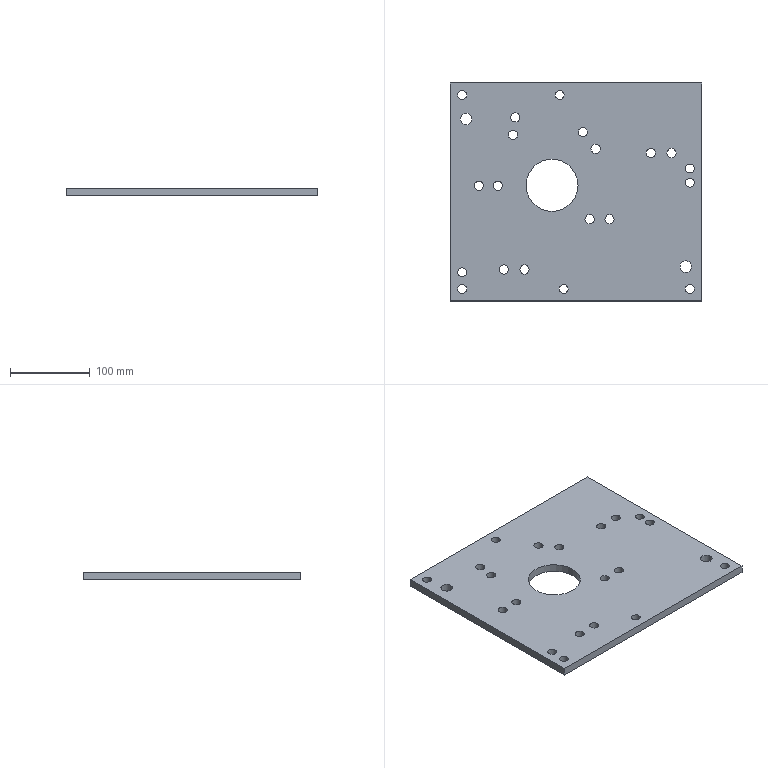Part | STEP file | lll_id3006_x_t | 1 solid | 29 faces | box 315 x 273 x 10 mm | volume 803171 mm3 | cylinder 23 | plane 6 | commonest cylinder face diameters 11.509 x12 11 x8 14.505 x2 65.2 x1
STEP:
#1=CARTESIAN_POINT('',(3327.121,-63.788,92.5));
#2=VERTEX_POINT('',#1);
#3=CARTESIAN_POINT('',(3321.367,-63.788,92.5));
#4=DIRECTION('',(0.,0.,1.));
#5=DIRECTION('',(1.,0.,0.));
#6=AXIS2_PLACEMENT_3D('',#3,#4,#5);
#7=CIRCLE('',#6,5.755);
#8=EDGE_CURVE('',#2,#2,#7,.T.);
#9=ORIENTED_EDGE('',*,*,#8,.F.);
#10=EDGE_LOOP('',(#9));
#11=FACE_BOUND('',#10,.T.);
#12=CARTESIAN_POINT('',(3315.612,-63.788,102.5));
#13=VERTEX_POINT('',#12);
#14=CARTESIAN_POINT('',(3321.367,-63.788,102.5));
#15=DIRECTION('',(0.,0.,-1.));
#16=DIRECTION('',(-1.,0.,0.));
#17=AXIS2_PLACEMENT_3D('',#14,#15,#16);
#18=CIRCLE('',#17,5.755);
#19=EDGE_CURVE('',#13,#13,#18,.T.);
#20=ORIENTED_EDGE('',*,*,#19,.F.);
#21=EDGE_LOOP('',(#20));
#22=FACE_BOUND('',#21,.T.);
#23=CARTESIAN_POINT('',(3321.367,-63.788,79.5));
#24=DIRECTION('',(0.,0.,1.));
#25=DIRECTION('',(1.,0.,0.));
#26=AXIS2_PLACEMENT_3D('',#23,#24,#25);
#27=CYLINDRICAL_SURFACE('',#26,5.755);
#28=ADVANCED_FACE('',(#11,#22),#27,.F.);
#29=CARTESIAN_POINT('',(3343.121,-84.788,92.5));
#30=VERTEX_POINT('',#29);
#31=CARTESIAN_POINT('',(3337.367,-84.788,92.5));
#32=DIRECTION('',(0.,0.,-1.));
#33=DIRECTION('',(1.,0.,0.));
#34=AXIS2_PLACEMENT_3D('',#31,#32,#33);
#35=CIRCLE('',#34,5.755);
#36=EDGE_CURVE('',#30,#30,#35,.T.);
#37=ORIENTED_EDGE('',*,*,#36,.T.);
#38=EDGE_LOOP('',(#37));
#39=FACE_BOUND('',#38,.T.);
#40=CARTESIAN_POINT('',(3331.612,-84.788,102.5));
#41=VERTEX_POINT('',#40);
#42=CARTESIAN_POINT('',(3337.367,-84.788,102.5));
#43=DIRECTION('',(0.,0.,-1.));
#44=DIRECTION('',(-1.,0.,0.));
#45=AXIS2_PLACEMENT_3D('',#42,#43,#44);
#46=CIRCLE('',#45,5.755);
#47=EDGE_CURVE('',#41,#41,#46,.T.);
#48=ORIENTED_EDGE('',*,*,#47,.F.);
#49=EDGE_LOOP('',(#48));
#50=FACE_BOUND('',#49,.T.);
#51=CARTESIAN_POINT('',(3337.367,-84.788,79.5));
#52=DIRECTION('',(0.,0.,1.));
#53=DIRECTION('',(1.,0.,0.));
#54=AXIS2_PLACEMENT_3D('',#51,#52,#53);
#55=CYLINDRICAL_SURFACE('',#54,5.755);
#56=ADVANCED_FACE('',(#39,#50),#55,.F.);
#57=CARTESIAN_POINT('',(3168.115,-47.288,102.5));
#58=VERTEX_POINT('',#57);
#59=CARTESIAN_POINT('',(3175.367,-47.288,102.5));
#60=DIRECTION('',(0.,0.,-1.));
#61=DIRECTION('',(-1.,0.,0.));
#62=AXIS2_PLACEMENT_3D('',#59,#60,#61);
#63=CIRCLE('',#62,7.253);
#64=EDGE_CURVE('',#58,#58,#63,.T.);
#65=ORIENTED_EDGE('',*,*,#64,.F.);
#66=EDGE_LOOP('',(#65));
#67=FACE_BOUND('',#66,.T.);
#68=CARTESIAN_POINT('',(3182.62,-47.288,92.5));
#69=VERTEX_POINT('',#68);
#70=CARTESIAN_POINT('',(3175.367,-47.288,92.5));
#71=DIRECTION('',(0.,0.,1.));
#72=DIRECTION('',(1.,0.,0.));
#73=AXIS2_PLACEMENT_3D('',#70,#71,#72);
#74=CIRCLE('',#73,7.253);
#75=EDGE_CURVE('',#69,#69,#74,.T.);
#76=ORIENTED_EDGE('',*,*,#75,.F.);
#77=EDGE_LOOP('',(#76));
#78=FACE_BOUND('',#77,.T.);
#79=CARTESIAN_POINT('',(3175.367,-47.288,92.5));
#80=DIRECTION('',(0.,0.,1.));
#81=DIRECTION('',(1.,0.,0.));
#82=AXIS2_PLACEMENT_3D('',#79,#80,#81);
#83=CYLINDRICAL_SURFACE('',#82,7.253);
#84=ADVANCED_FACE('',(#67,#78),#83,.F.);
#85=CARTESIAN_POINT('',(3324.113,-172.788,102.5));
#86=VERTEX_POINT('',#85);
#87=CARTESIAN_POINT('',(3329.867,-172.788,102.5));
#88=DIRECTION('',(0.,0.,1.));
#89=DIRECTION('',(-1.,0.,0.));
#90=AXIS2_PLACEMENT_3D('',#87,#88,#89);
#91=CIRCLE('',#90,5.755);
#92=EDGE_CURVE('',#86,#86,#91,.T.);
#93=ORIENTED_EDGE('',*,*,#92,.T.);
#94=EDGE_LOOP('',(#93));
#95=FACE_BOUND('',#94,.T.);
#96=CARTESIAN_POINT('',(3335.622,-172.788,92.5));
#97=VERTEX_POINT('',#96);
#98=CARTESIAN_POINT('',(3329.867,-172.788,92.5));
#99=DIRECTION('',(0.,0.,1.));
#100=DIRECTION('',(1.,0.,0.));
#101=AXIS2_PLACEMENT_3D('',#98,#99,#100);
#102=CIRCLE('',#101,5.755);
#103=EDGE_CURVE('',#97,#97,#102,.T.);
#104=ORIENTED_EDGE('',*,*,#103,.F.);
#105=EDGE_LOOP('',(#104));
#106=FACE_BOUND('',#105,.T.);
#107=CARTESIAN_POINT('',(3329.867,-172.788,92.5));
#108=DIRECTION('',(0.,0.,1.));
#109=DIRECTION('',(1.,0.,0.));
#110=AXIS2_PLACEMENT_3D('',#107,#108,#109);
#111=CYLINDRICAL_SURFACE('',#110,5.755);
#112=ADVANCED_FACE('',(#95,#106),#111,.F.);
#113=CARTESIAN_POINT('',(3216.612,-235.788,102.5));
#114=VERTEX_POINT('',#113);
#115=CARTESIAN_POINT('',(3222.367,-235.788,102.5));
#116=DIRECTION('',(0.,0.,-1.));
#117=DIRECTION('',(-1.,0.,0.));
#118=AXIS2_PLACEMENT_3D('',#115,#116,#117);
#119=CIRCLE('',#118,5.755);
#120=EDGE_CURVE('',#114,#114,#119,.T.);
#121=ORIENTED_EDGE('',*,*,#120,.F.);
#122=EDGE_LOOP('',(#121));
#123=FACE_BOUND('',#122,.T.);
#124=CARTESIAN_POINT('',(3228.121,-235.788,92.5));
#125=VERTEX_POINT('',#124);
#126=CARTESIAN_POINT('',(3222.367,-235.788,92.5));
#127=DIRECTION('',(0.,0.,1.));
#128=DIRECTION('',(1.,0.,0.));
#129=AXIS2_PLACEMENT_3D('',#126,#127,#128);
#130=CIRCLE('',#129,5.755);
#131=EDGE_CURVE('',#125,#125,#130,.T.);
#132=ORIENTED_EDGE('',*,*,#131,.F.);
#133=EDGE_LOOP('',(#132));
#134=FACE_BOUND('',#133,.T.);
#135=CARTESIAN_POINT('',(3222.367,-235.788,92.5));
#136=DIRECTION('',(0.,0.,1.));
#137=DIRECTION('',(1.,0.,0.));
#138=AXIS2_PLACEMENT_3D('',#135,#136,#137);
#139=CYLINDRICAL_SURFACE('',#138,5.755);
#140=ADVANCED_FACE('',(#123,#134),#139,.F.);
#141=CARTESIAN_POINT('',(3209.245,-131.,102.5));
#142=VERTEX_POINT('',#141);
#143=CARTESIAN_POINT('',(3215.,-131.,102.5));
#144=DIRECTION('',(0.,0.,1.));
#145=DIRECTION('',(-1.,0.,0.));
#146=AXIS2_PLACEMENT_3D('',#143,#144,#145);
#147=CIRCLE('',#146,5.755);
#148=EDGE_CURVE('',#142,#142,#147,.T.);
#149=ORIENTED_EDGE('',*,*,#148,.T.);
#150=EDGE_LOOP('',(#149));
#151=FACE_BOUND('',#150,.T.);
#152=CARTESIAN_POINT('',(3220.755,-131.,92.5));
#153=VERTEX_POINT('',#152);
#154=CARTESIAN_POINT('',(3215.,-131.,92.5));
#155=DIRECTION('',(0.,0.,1.));
#156=DIRECTION('',(1.,0.,0.));
#157=AXIS2_PLACEMENT_3D('',#154,#155,#156);
#158=CIRCLE('',#157,5.755);
#159=EDGE_CURVE('',#153,#153,#158,.T.);
#160=ORIENTED_EDGE('',*,*,#159,.F.);
#161=EDGE_LOOP('',(#160));
#162=FACE_BOUND('',#161,.T.);
#163=CARTESIAN_POINT('',(3215.,-131.,92.5));
#164=DIRECTION('',(0.,0.,1.));
#165=DIRECTION('',(1.,0.,0.));
#166=AXIS2_PLACEMENT_3D('',#163,#164,#165);
#167=CYLINDRICAL_SURFACE('',#166,5.755);
#168=ADVANCED_FACE('',(#151,#162),#167,.F.);
#169=CARTESIAN_POINT('',(3400.746,-90.,102.5));
#170=VERTEX_POINT('',#169);
#171=CARTESIAN_POINT('',(3406.5,-90.,102.5));
#172=DIRECTION('',(0.,0.,1.));
#173=DIRECTION('',(-1.,0.,0.));
#174=AXIS2_PLACEMENT_3D('',#171,#172,#173);
#175=CIRCLE('',#174,5.755);
#176=EDGE_CURVE('',#170,#170,#175,.T.);
#177=ORIENTED_EDGE('',*,*,#176,.T.);
#178=EDGE_LOOP('',(#177));
#179=FACE_BOUND('',#178,.T.);
#180=CARTESIAN_POINT('',(3412.255,-90.,92.5));
#181=VERTEX_POINT('',#180);
#182=CARTESIAN_POINT('',(3406.5,-90.,92.5));
#183=DIRECTION('',(0.,0.,1.));
#184=DIRECTION('',(1.,0.,0.));
#185=AXIS2_PLACEMENT_3D('',#182,#183,#184);
#186=CIRCLE('',#185,5.755);
#187=EDGE_CURVE('',#181,#181,#186,.T.);
#188=ORIENTED_EDGE('',*,*,#187,.F.);
#189=EDGE_LOOP('',(#188));
#190=FACE_BOUND('',#189,.T.);
#191=CARTESIAN_POINT('',(3406.5,-90.,92.5));
#192=DIRECTION('',(0.,0.,1.));
#193=DIRECTION('',(1.,0.,0.));
#194=AXIS2_PLACEMENT_3D('',#191,#192,#193);
#195=CYLINDRICAL_SURFACE('',#194,5.755);
#196=ADVANCED_FACE('',(#179,#190),#195,.F.);
#197=CARTESIAN_POINT('',(3228.222,-67.288,102.5));
#198=VERTEX_POINT('',#197);
#199=CARTESIAN_POINT('',(3233.977,-67.288,102.5));
#200=DIRECTION('',(0.,0.,1.));
#201=DIRECTION('',(-1.,0.,0.));
#202=AXIS2_PLACEMENT_3D('',#199,#200,#201);
#203=CIRCLE('',#202,5.755);
#204=EDGE_CURVE('',#198,#198,#203,.T.);
#205=ORIENTED_EDGE('',*,*,#204,.T.);
#206=EDGE_LOOP('',(#205));
#207=FACE_BOUND('',#206,.T.);
#208=CARTESIAN_POINT('',(3239.731,-67.288,92.5));
#209=VERTEX_POINT('',#208);
#210=CARTESIAN_POINT('',(3233.977,-67.288,92.5));
#211=DIRECTION('',(0.,0.,1.));
#212=DIRECTION('',(1.,0.,0.));
#213=AXIS2_PLACEMENT_3D('',#210,#211,#212);
#214=CIRCLE('',#213,5.755);
#215=EDGE_CURVE('',#209,#209,#214,.T.);
#216=ORIENTED_EDGE('',*,*,#215,.F.);
#217=EDGE_LOOP('',(#216));
#218=FACE_BOUND('',#217,.T.);
#219=CARTESIAN_POINT('',(3233.977,-67.288,92.5));
#220=DIRECTION('',(0.,0.,1.));
#221=DIRECTION('',(1.,0.,0.));
#222=AXIS2_PLACEMENT_3D('',#219,#220,#221);
#223=CYLINDRICAL_SURFACE('',#222,5.755);
#224=ADVANCED_FACE('',(#207,#218),#223,.F.);
#225=CARTESIAN_POINT('',(3449.867,-127.288,102.5));
#226=VERTEX_POINT('',#225);
#227=CARTESIAN_POINT('',(3455.367,-127.288,102.5));
#228=DIRECTION('',(0.,0.,-1.));
#229=DIRECTION('',(-1.,0.,0.));
#230=AXIS2_PLACEMENT_3D('',#227,#228,#229);
#231=CIRCLE('',#230,5.5);
#232=EDGE_CURVE('',#226,#226,#231,.T.);
#233=ORIENTED_EDGE('',*,*,#232,.F.);
#234=EDGE_LOOP('',(#233));
#235=FACE_BOUND('',#234,.T.);
#236=CARTESIAN_POINT('',(3460.867,-127.288,92.5));
#237=VERTEX_POINT('',#236);
#238=CARTESIAN_POINT('',(3455.367,-127.288,92.5));
#239=DIRECTION('',(0.,0.,1.));
#240=DIRECTION('',(1.,0.,0.));
#241=AXIS2_PLACEMENT_3D('',#238,#239,#240);
#242=CIRCLE('',#241,5.5);
#243=EDGE_CURVE('',#237,#237,#242,.T.);
#244=ORIENTED_EDGE('',*,*,#243,.F.);
#245=EDGE_LOOP('',(#244));
#246=FACE_BOUND('',#245,.T.);
#247=CARTESIAN_POINT('',(3455.367,-127.288,92.5));
#248=DIRECTION('',(0.,0.,-1.));
#249=DIRECTION('',(1.,0.,0.));
#250=AXIS2_PLACEMENT_3D('',#247,#248,#249);
#251=CYLINDRICAL_SURFACE('',#250,5.5);
#252=ADVANCED_FACE('',(#235,#246),#251,.F.);
#253=CARTESIAN_POINT('',(3164.867,-239.288,102.5));
#254=VERTEX_POINT('',#253);
#255=CARTESIAN_POINT('',(3170.367,-239.288,102.5));
#256=DIRECTION('',(0.,0.,-1.));
#257=DIRECTION('',(-1.,0.,0.));
#258=AXIS2_PLACEMENT_3D('',#255,#256,#257);
#259=CIRCLE('',#258,5.5);
#260=EDGE_CURVE('',#254,#254,#259,.T.);
#261=ORIENTED_EDGE('',*,*,#260,.F.);
#262=EDGE_LOOP('',(#261));
#263=FACE_BOUND('',#262,.T.);
#264=CARTESIAN_POINT('',(3175.867,-239.288,92.5));
#265=VERTEX_POINT('',#264);
#266=CARTESIAN_POINT('',(3170.367,-239.288,92.5));
#267=DIRECTION('',(0.,0.,1.));
#268=DIRECTION('',(1.,0.,0.));
#269=AXIS2_PLACEMENT_3D('',#266,#267,#268);
#270=CIRCLE('',#269,5.5);
#271=EDGE_CURVE('',#265,#265,#270,.T.);
#272=ORIENTED_EDGE('',*,*,#271,.F.);
#273=EDGE_LOOP('',(#272));
#274=FACE_BOUND('',#273,.T.);
#275=CARTESIAN_POINT('',(3170.367,-239.288,92.5));
#276=DIRECTION('',(0.,0.,-1.));
#277=DIRECTION('',(1.,0.,0.));
#278=AXIS2_PLACEMENT_3D('',#275,#276,#277);
#279=CYLINDRICAL_SURFACE('',#278,5.5);
#280=ADVANCED_FACE('',(#263,#274),#279,.F.);
#281=CARTESIAN_POINT('',(3449.867,-109.288,102.5));
#282=VERTEX_POINT('',#281);
#283=CARTESIAN_POINT('',(3455.367,-109.288,102.5));
#284=DIRECTION('',(0.,0.,1.));
#285=DIRECTION('',(-1.,0.,0.));
#286=AXIS2_PLACEMENT_3D('',#283,#284,#285);
#287=CIRCLE('',#286,5.5);
#288=EDGE_CURVE('',#282,#282,#287,.T.);
#289=ORIENTED_EDGE('',*,*,#288,.T.);
#290=EDGE_LOOP('',(#289));
#291=FACE_BOUND('',#290,.T.);
#292=CARTESIAN_POINT('',(3449.867,-109.288,92.5));
#293=VERTEX_POINT('',#292);
#294=CARTESIAN_POINT('',(3455.367,-109.288,92.5));
#295=DIRECTION('',(0.,0.,1.));
#296=DIRECTION('',(-1.,0.,0.));
#297=AXIS2_PLACEMENT_3D('',#294,#295,#296);
#298=CIRCLE('',#297,5.5);
#299=EDGE_CURVE('',#293,#293,#298,.T.);
#300=ORIENTED_EDGE('',*,*,#299,.F.);
#301=EDGE_LOOP('',(#300));
#302=FACE_BOUND('',#301,.T.);
#303=CARTESIAN_POINT('',(3455.367,-109.288,92.5));
#304=DIRECTION('',(0.,0.,-1.));
#305=DIRECTION('',(1.,0.,0.));
#306=AXIS2_PLACEMENT_3D('',#303,#304,#305);
#307=CYLINDRICAL_SURFACE('',#306,5.5);
#308=ADVANCED_FACE('',(#291,#302),#307,.F.);
#309=CARTESIAN_POINT('',(3164.867,-17.288,102.5));
#310=VERTEX_POINT('',#309);
#311=CARTESIAN_POINT('',(3170.367,-17.288,102.5));
#312=DIRECTION('',(0.,0.,1.));
#313=DIRECTION('',(-1.,0.,0.));
#314=AXIS2_PLACEMENT_3D('',#311,#312,#313);
#315=CIRCLE('',#314,5.5);
#316=EDGE_CURVE('',#310,#310,#315,.T.);
#317=ORIENTED_EDGE('',*,*,#316,.T.);
#318=EDGE_LOOP('',(#317));
#319=FACE_BOUND('',#318,.T.);
#320=CARTESIAN_POINT('',(3164.867,-17.288,92.5));
#321=VERTEX_POINT('',#320);
#322=CARTESIAN_POINT('',(3170.367,-17.288,92.5));
#323=DIRECTION('',(0.,0.,1.));
#324=DIRECTION('',(-1.,0.,0.));
#325=AXIS2_PLACEMENT_3D('',#322,#323,#324);
#326=CIRCLE('',#325,5.5);
#327=EDGE_CURVE('',#321,#321,#326,.T.);
#328=ORIENTED_EDGE('',*,*,#327,.F.);
#329=EDGE_LOOP('',(#328));
#330=FACE_BOUND('',#329,.T.);
#331=CARTESIAN_POINT('',(3170.367,-17.288,92.5));
#332=DIRECTION('',(0.,0.,-1.));
#333=DIRECTION('',(1.,0.,0.));
#334=AXIS2_PLACEMENT_3D('',#331,#332,#333);
#335=CYLINDRICAL_SURFACE('',#334,5.5);
#336=ADVANCED_FACE('',(#319,#330),#335,.F.);
#337=CARTESIAN_POINT('',(3155.367,-275.288,102.5));
#338=VERTEX_POINT('',#337);
#339=CARTESIAN_POINT('',(3155.367,-275.288,92.5));
#340=VERTEX_POINT('',#339);
#341=CARTESIAN_POINT('',(3155.367,-275.288,92.5));
#342=DIRECTION('',(0.,0.,-1.));
#343=VECTOR('',#342,1.);
#344=LINE('',#341,#343);
#345=EDGE_CURVE('',#338,#340,#344,.T.);
#346=ORIENTED_EDGE('',*,*,#345,.F.);
#347=CARTESIAN_POINT('',(3155.367,-2.288,102.5));
#348=VERTEX_POINT('',#347);
#349=CARTESIAN_POINT('',(3155.367,-166.13,102.5));
#350=DIRECTION('',(0.,-1.,0.));
#351=VECTOR('',#350,1.);
#352=LINE('',#349,#351);
#353=EDGE_CURVE('',#348,#338,#352,.T.);
#354=ORIENTED_EDGE('',*,*,#353,.F.);
#355=CARTESIAN_POINT('',(3155.367,-2.288,92.5));
#356=VERTEX_POINT('',#355);
#357=CARTESIAN_POINT('',(3155.367,-2.288,92.5));
#358=DIRECTION('',(0.,0.,-1.));
#359=VECTOR('',#358,1.);
#360=LINE('',#357,#359);
#361=EDGE_CURVE('',#348,#356,#360,.T.);
#362=ORIENTED_EDGE('',*,*,#361,.T.);
#363=CARTESIAN_POINT('',(3155.367,-166.13,92.5));
#364=DIRECTION('',(0.,-1.,0.));
#365=VECTOR('',#364,1.);
#366=LINE('',#363,#365);
#367=EDGE_CURVE('',#356,#340,#366,.T.);
#368=ORIENTED_EDGE('',*,*,#367,.T.);
#369=EDGE_LOOP('',(#346,#354,#362,#368));
#370=FACE_OUTER_BOUND('',#369,.T.);
#371=CARTESIAN_POINT('',(3155.367,-166.13,92.5));
#372=DIRECTION('',(-1.,0.,0.));
#373=DIRECTION('',(0.,-1.,0.));
#374=AXIS2_PLACEMENT_3D('',#371,#372,#373);
#375=PLANE('',#374);
#376=ADVANCED_FACE('',(#370),#375,.T.);
#377=CARTESIAN_POINT('',(3470.367,-275.288,102.5));
#378=VERTEX_POINT('',#377);
#379=CARTESIAN_POINT('',(3470.367,-275.288,92.5));
#380=VERTEX_POINT('',#379);
#381=CARTESIAN_POINT('',(3470.367,-275.288,92.5));
#382=DIRECTION('',(0.,0.,-1.));
#383=VECTOR('',#382,1.);
#384=LINE('',#381,#383);
#385=EDGE_CURVE('',#378,#380,#384,.T.);
#386=ORIENTED_EDGE('',*,*,#385,.F.);
#387=CARTESIAN_POINT('',(3227.867,-275.288,102.5));
#388=DIRECTION('',(1.,0.,0.));
#389=VECTOR('',#388,1.);
#390=LINE('',#387,#389);
#391=EDGE_CURVE('',#338,#378,#390,.T.);
#392=ORIENTED_EDGE('',*,*,#391,.F.);
#393=ORIENTED_EDGE('',*,*,#345,.T.);
#394=CARTESIAN_POINT('',(3227.867,-275.288,92.5));
#395=DIRECTION('',(-1.,0.,0.));
#396=VECTOR('',#395,1.);
#397=LINE('',#394,#396);
#398=EDGE_CURVE('',#380,#340,#397,.T.);
#399=ORIENTED_EDGE('',*,*,#398,.F.);
#400=EDGE_LOOP('',(#386,#392,#393,#399));
#401=FACE_OUTER_BOUND('',#400,.T.);
#402=CARTESIAN_POINT('',(3227.867,-275.288,92.5));
#403=DIRECTION('',(0.,1.,0.));
#404=DIRECTION('',(-1.,0.,0.));
#405=AXIS2_PLACEMENT_3D('',#402,#403,#404);
#406=PLANE('',#405);
#407=ADVANCED_FACE('',(#401),#406,.F.);
#408=CARTESIAN_POINT('',(3470.367,-2.288,102.5));
#409=VERTEX_POINT('',#408);
#410=CARTESIAN_POINT('',(3470.367,-2.288,92.5));
#411=VERTEX_POINT('',#410);
#412=CARTESIAN_POINT('',(3470.367,-2.288,92.5));
#413=DIRECTION('',(0.,0.,-1.));
#414=VECTOR('',#413,1.);
#415=LINE('',#412,#414);
#416=EDGE_CURVE('',#409,#411,#415,.T.);
#417=ORIENTED_EDGE('',*,*,#416,.F.);
#418=CARTESIAN_POINT('',(3470.367,-195.288,102.5));
#419=DIRECTION('',(0.,-1.,0.));
#420=VECTOR('',#419,1.);
#421=LINE('',#418,#420);
#422=EDGE_CURVE('',#409,#378,#421,.T.);
#423=ORIENTED_EDGE('',*,*,#422,.T.);
#424=ORIENTED_EDGE('',*,*,#385,.T.);
#425=CARTESIAN_POINT('',(3470.367,-195.288,92.5));
#426=DIRECTION('',(0.,-1.,0.));
#427=VECTOR('',#426,1.);
#428=LINE('',#425,#427);
#429=EDGE_CURVE('',#411,#380,#428,.T.);
#430=ORIENTED_EDGE('',*,*,#429,.F.);
#431=EDGE_LOOP('',(#417,#423,#424,#430));
#432=FACE_OUTER_BOUND('',#431,.T.);
#433=CARTESIAN_POINT('',(3470.367,-195.288,92.5));
#434=DIRECTION('',(-1.,0.,0.));
#435=DIRECTION('',(0.,-1.,0.));
#436=AXIS2_PLACEMENT_3D('',#433,#434,#435);
#437=PLANE('',#436);
#438=ADVANCED_FACE('',(#432),#437,.F.);
#439=ORIENTED_EDGE('',*,*,#361,.F.);
#440=CARTESIAN_POINT('',(3227.867,-2.288,102.5));
#441=DIRECTION('',(1.,0.,0.));
#442=VECTOR('',#441,1.);
#443=LINE('',#440,#442);
#444=EDGE_CURVE('',#348,#409,#443,.T.);
#445=ORIENTED_EDGE('',*,*,#444,.T.);
#446=ORIENTED_EDGE('',*,*,#416,.T.);
#447=CARTESIAN_POINT('',(3227.867,-2.288,92.5));
#448=DIRECTION('',(1.,0.,0.));
#449=VECTOR('',#448,1.);
#450=LINE('',#447,#449);
#451=EDGE_CURVE('',#356,#411,#450,.T.);
#452=ORIENTED_EDGE('',*,*,#451,.F.);
#453=EDGE_LOOP('',(#439,#445,#446,#452));
#454=FACE_OUTER_BOUND('',#453,.T.);
#455=CARTESIAN_POINT('',(3227.867,-2.288,92.5));
#456=DIRECTION('',(0.,-1.,0.));
#457=DIRECTION('',(1.,0.,0.));
#458=AXIS2_PLACEMENT_3D('',#455,#456,#457);
#459=PLANE('',#458);
#460=ADVANCED_FACE('',(#454),#459,.F.);
#461=CARTESIAN_POINT('',(3164.867,-260.288,102.5));
#462=VERTEX_POINT('',#461);
#463=CARTESIAN_POINT('',(3170.367,-260.288,102.5));
#464=DIRECTION('',(0.,0.,-1.));
#465=DIRECTION('',(-1.,0.,0.));
#466=AXIS2_PLACEMENT_3D('',#463,#464,#465);
#467=CIRCLE('',#466,5.5);
#468=EDGE_CURVE('',#462,#462,#467,.T.);
#469=ORIENTED_EDGE('',*,*,#468,.F.);
#470=EDGE_LOOP('',(#469));
#471=FACE_BOUND('',#470,.T.);
#472=CARTESIAN_POINT('',(3164.867,-260.288,92.5));
#473=VERTEX_POINT('',#472);
#474=CARTESIAN_POINT('',(3170.367,-260.288,92.5));
#475=DIRECTION('',(0.,0.,1.));
#476=DIRECTION('',(-1.,0.,0.));
#477=AXIS2_PLACEMENT_3D('',#474,#475,#476);
#478=CIRCLE('',#477,5.5);
#479=EDGE_CURVE('',#473,#473,#478,.T.);
#480=ORIENTED_EDGE('',*,*,#479,.F.);
#481=EDGE_LOOP('',(#480));
#482=FACE_BOUND('',#481,.T.);
#483=CARTESIAN_POINT('',(3170.367,-260.288,92.5));
#484=DIRECTION('',(0.,0.,-1.));
#485=DIRECTION('',(1.,0.,0.));
#486=AXIS2_PLACEMENT_3D('',#483,#484,#485);
#487=CYLINDRICAL_SURFACE('',#486,5.5);
#488=ADVANCED_FACE('',(#471,#482),#487,.F.);
#489=CARTESIAN_POINT('',(3449.867,-260.288,102.5));
#490=VERTEX_POINT('',#489);
#491=CARTESIAN_POINT('',(3455.367,-260.288,102.5));
#492=DIRECTION('',(0.,0.,-1.));
#493=DIRECTION('',(-1.,0.,0.));
#494=AXIS2_PLACEMENT_3D('',#491,#492,#493);
#495=CIRCLE('',#494,5.5);
#496=EDGE_CURVE('',#490,#490,#495,.T.);
#497=ORIENTED_EDGE('',*,*,#496,.F.);
#498=EDGE_LOOP('',(#497));
#499=FACE_BOUND('',#498,.T.);
#500=CARTESIAN_POINT('',(3449.867,-260.288,92.5));
#501=VERTEX_POINT('',#500);
#502=CARTESIAN_POINT('',(3455.367,-260.288,92.5));
#503=DIRECTION('',(0.,0.,-1.));
#504=DIRECTION('',(-1.,0.,0.));
#505=AXIS2_PLACEMENT_3D('',#502,#503,#504);
#506=CIRCLE('',#505,5.5);
#507=EDGE_CURVE('',#501,#501,#506,.T.);
#508=ORIENTED_EDGE('',*,*,#507,.T.);
#509=EDGE_LOOP('',(#508));
#510=FACE_BOUND('',#509,.T.);
#511=CARTESIAN_POINT('',(3455.367,-260.288,92.5));
#512=DIRECTION('',(0.,0.,-1.));
#513=DIRECTION('',(1.,0.,0.));
#514=AXIS2_PLACEMENT_3D('',#511,#512,#513);
#515=CYLINDRICAL_SURFACE('',#514,5.5);
#516=ADVANCED_FACE('',(#499,#510),#515,.F.);
#517=CARTESIAN_POINT('',(3291.867,-260.288,102.5));
#518=VERTEX_POINT('',#517);
#519=CARTESIAN_POINT('',(3297.367,-260.288,102.5));
#520=DIRECTION('',(0.,0.,1.));
#521=DIRECTION('',(-1.,0.,0.));
#522=AXIS2_PLACEMENT_3D('',#519,#520,#521);
#523=CIRCLE('',#522,5.5);
#524=EDGE_CURVE('',#518,#518,#523,.T.);
#525=ORIENTED_EDGE('',*,*,#524,.T.);
#526=EDGE_LOOP('',(#525));
#527=FACE_BOUND('',#526,.T.);
#528=CARTESIAN_POINT('',(3291.867,-260.288,92.5));
#529=VERTEX_POINT('',#528);
#530=CARTESIAN_POINT('',(3297.367,-260.288,92.5));
#531=DIRECTION('',(0.,0.,-1.));
#532=DIRECTION('',(-1.,0.,0.));
#533=AXIS2_PLACEMENT_3D('',#530,#531,#532);
#534=CIRCLE('',#533,5.5);
#535=EDGE_CURVE('',#529,#529,#534,.T.);
#536=ORIENTED_EDGE('',*,*,#535,.T.);
#537=EDGE_LOOP('',(#536));
#538=FACE_BOUND('',#537,.T.);
#539=CARTESIAN_POINT('',(3297.367,-260.288,92.5));
#540=DIRECTION('',(0.,0.,-1.));
#541=DIRECTION('',(1.,0.,0.));
#542=AXIS2_PLACEMENT_3D('',#539,#540,#541);
#543=CYLINDRICAL_SURFACE('',#542,5.5);
#544=ADVANCED_FACE('',(#527,#538),#543,.F.);
#545=CARTESIAN_POINT('',(3286.867,-17.288,102.5));
#546=VERTEX_POINT('',#545);
#547=CARTESIAN_POINT('',(3292.367,-17.288,102.5));
#548=DIRECTION('',(0.,0.,1.));
#549=DIRECTION('',(-1.,0.,0.));
#550=AXIS2_PLACEMENT_3D('',#547,#548,#549);
#551=CIRCLE('',#550,5.5);
#552=EDGE_CURVE('',#546,#546,#551,.T.);
#553=ORIENTED_EDGE('',*,*,#552,.T.);
#554=EDGE_LOOP('',(#553));
#555=FACE_BOUND('',#554,.T.);
#556=CARTESIAN_POINT('',(3286.867,-17.288,92.5));
#557=VERTEX_POINT('',#556);
#558=CARTESIAN_POINT('',(3292.367,-17.288,92.5));
#559=DIRECTION('',(0.,0.,-1.));
#560=DIRECTION('',(-1.,0.,0.));
#561=AXIS2_PLACEMENT_3D('',#558,#559,#560);
#562=CIRCLE('',#561,5.5);
#563=EDGE_CURVE('',#557,#557,#562,.T.);
#564=ORIENTED_EDGE('',*,*,#563,.T.);
#565=EDGE_LOOP('',(#564));
#566=FACE_BOUND('',#565,.T.);
#567=CARTESIAN_POINT('',(3292.367,-17.288,92.5));
#568=DIRECTION('',(0.,0.,-1.));
#569=DIRECTION('',(1.,0.,0.));
#570=AXIS2_PLACEMENT_3D('',#567,#568,#569);
#571=CYLINDRICAL_SURFACE('',#570,5.5);
#572=ADVANCED_FACE('',(#555,#566),#571,.F.);
#573=CARTESIAN_POINT('',(3443.115,-232.288,102.5));
#574=VERTEX_POINT('',#573);
#575=CARTESIAN_POINT('',(3450.367,-232.288,102.5));
#576=DIRECTION('',(0.,0.,-1.));
#577=DIRECTION('',(-1.,0.,0.));
#578=AXIS2_PLACEMENT_3D('',#575,#576,#577);
#579=CIRCLE('',#578,7.253);
#580=EDGE_CURVE('',#574,#574,#579,.T.);
#581=ORIENTED_EDGE('',*,*,#580,.F.);
#582=EDGE_LOOP('',(#581));
#583=FACE_BOUND('',#582,.T.);
#584=CARTESIAN_POINT('',(3457.62,-232.288,92.5));
#585=VERTEX_POINT('',#584);
#586=CARTESIAN_POINT('',(3450.367,-232.288,92.5));
#587=DIRECTION('',(0.,0.,1.));
#588=DIRECTION('',(1.,0.,0.));
#589=AXIS2_PLACEMENT_3D('',#586,#587,#588);
#590=CIRCLE('',#589,7.253);
#591=EDGE_CURVE('',#585,#585,#590,.T.);
#592=ORIENTED_EDGE('',*,*,#591,.F.);
#593=EDGE_LOOP('',(#592));
#594=FACE_BOUND('',#593,.T.);
#595=CARTESIAN_POINT('',(3450.367,-232.288,92.5));
#596=DIRECTION('',(0.,0.,1.));
#597=DIRECTION('',(1.,0.,0.));
#598=AXIS2_PLACEMENT_3D('',#595,#596,#597);
#599=CYLINDRICAL_SURFACE('',#598,7.253);
#600=ADVANCED_FACE('',(#583,#594),#599,.F.);
#601=CARTESIAN_POINT('',(3250.256,-130.4,102.5));
#602=VERTEX_POINT('',#601);
#603=CARTESIAN_POINT('',(3282.856,-130.4,102.5));
#604=DIRECTION('',(0.,0.,-1.));
#605=DIRECTION('',(-1.,0.,0.));
#606=AXIS2_PLACEMENT_3D('',#603,#604,#605);
#607=CIRCLE('',#606,32.6);
#608=EDGE_CURVE('',#602,#602,#607,.T.);
#609=ORIENTED_EDGE('',*,*,#608,.F.);
#610=EDGE_LOOP('',(#609));
#611=FACE_BOUND('',#610,.T.);
#612=CARTESIAN_POINT('',(3315.456,-130.4,92.5));
#613=VERTEX_POINT('',#612);
#614=CARTESIAN_POINT('',(3282.856,-130.4,92.5));
#615=DIRECTION('',(0.,0.,1.));
#616=DIRECTION('',(1.,0.,0.));
#617=AXIS2_PLACEMENT_3D('',#614,#615,#616);
#618=CIRCLE('',#617,32.6);
#619=EDGE_CURVE('',#613,#613,#618,.T.);
#620=ORIENTED_EDGE('',*,*,#619,.F.);
#621=EDGE_LOOP('',(#620));
#622=FACE_BOUND('',#621,.T.);
#623=CARTESIAN_POINT('',(3282.856,-130.4,-337.5));
#624=DIRECTION('',(0.,0.,1.));
#625=DIRECTION('',(1.,0.,0.));
#626=AXIS2_PLACEMENT_3D('',#623,#624,#625);
#627=CYLINDRICAL_SURFACE('',#626,32.6);
#628=ADVANCED_FACE('',(#611,#622),#627,.F.);
#629=CARTESIAN_POINT('',(3349.112,-172.788,102.5));
#630=VERTEX_POINT('',#629);
#631=CARTESIAN_POINT('',(3354.867,-172.788,102.5));
#632=DIRECTION('',(0.,0.,-1.));
#633=DIRECTION('',(-1.,0.,0.));
#634=AXIS2_PLACEMENT_3D('',#631,#632,#633);
#635=CIRCLE('',#634,5.755);
#636=EDGE_CURVE('',#630,#630,#635,.T.);
#637=ORIENTED_EDGE('',*,*,#636,.F.);
#638=EDGE_LOOP('',(#637));
#639=FACE_BOUND('',#638,.T.);
#640=CARTESIAN_POINT('',(3360.621,-172.788,92.5));
#641=VERTEX_POINT('',#640);
#642=CARTESIAN_POINT('',(3354.867,-172.788,92.5));
#643=DIRECTION('',(0.,0.,1.));
#644=DIRECTION('',(1.,0.,0.));
#645=AXIS2_PLACEMENT_3D('',#642,#643,#644);
#646=CIRCLE('',#645,5.755);
#647=EDGE_CURVE('',#641,#641,#646,.T.);
#648=ORIENTED_EDGE('',*,*,#647,.F.);
#649=EDGE_LOOP('',(#648));
#650=FACE_BOUND('',#649,.T.);
#651=CARTESIAN_POINT('',(3354.867,-172.788,92.5));
#652=DIRECTION('',(0.,0.,1.));
#653=DIRECTION('',(1.,0.,0.));
#654=AXIS2_PLACEMENT_3D('',#651,#652,#653);
#655=CYLINDRICAL_SURFACE('',#654,5.755);
#656=ADVANCED_FACE('',(#639,#650),#655,.F.);
#657=CARTESIAN_POINT('',(3242.612,-235.788,102.5));
#658=VERTEX_POINT('',#657);
#659=CARTESIAN_POINT('',(3248.367,-235.788,102.5));
#660=DIRECTION('',(0.,0.,-1.));
#661=DIRECTION('',(-1.,0.,0.));
#662=AXIS2_PLACEMENT_3D('',#659,#660,#661);
#663=CIRCLE('',#662,5.755);
#664=EDGE_CURVE('',#658,#658,#663,.T.);
#665=ORIENTED_EDGE('',*,*,#664,.F.);
#666=EDGE_LOOP('',(#665));
#667=FACE_BOUND('',#666,.T.);
#668=CARTESIAN_POINT('',(3254.121,-235.788,92.5));
#669=VERTEX_POINT('',#668);
#670=CARTESIAN_POINT('',(3248.367,-235.788,92.5));
#671=DIRECTION('',(0.,0.,1.));
#672=DIRECTION('',(1.,0.,0.));
#673=AXIS2_PLACEMENT_3D('',#670,#671,#672);
#674=CIRCLE('',#673,5.755);
#675=EDGE_CURVE('',#669,#669,#674,.T.);
#676=ORIENTED_EDGE('',*,*,#675,.F.);
#677=EDGE_LOOP('',(#676));
#678=FACE_BOUND('',#677,.T.);
#679=CARTESIAN_POINT('',(3248.367,-235.788,92.5));
#680=DIRECTION('',(0.,0.,1.));
#681=DIRECTION('',(1.,0.,0.));
#682=AXIS2_PLACEMENT_3D('',#679,#680,#681);
#683=CYLINDRICAL_SURFACE('',#682,5.755);
#684=ADVANCED_FACE('',(#667,#678),#683,.F.);
#685=CARTESIAN_POINT('',(3426.746,-90.,102.5));
#686=VERTEX_POINT('',#685);
#687=CARTESIAN_POINT('',(3432.5,-90.,102.5));
#688=DIRECTION('',(0.,0.,-1.));
#689=DIRECTION('',(-1.,0.,0.));
#690=AXIS2_PLACEMENT_3D('',#687,#688,#689);
#691=CIRCLE('',#690,5.755);
#692=EDGE_CURVE('',#686,#686,#691,.T.);
#693=ORIENTED_EDGE('',*,*,#692,.F.);
#694=EDGE_LOOP('',(#693));
#695=FACE_BOUND('',#694,.T.);
#696=CARTESIAN_POINT('',(3438.255,-90.,92.5));
#697=VERTEX_POINT('',#696);
#698=CARTESIAN_POINT('',(3432.5,-90.,92.5));
#699=DIRECTION('',(0.,0.,1.));
#700=DIRECTION('',(1.,0.,0.));
#701=AXIS2_PLACEMENT_3D('',#698,#699,#700);
#702=CIRCLE('',#701,5.755);
#703=EDGE_CURVE('',#697,#697,#702,.T.);
#704=ORIENTED_EDGE('',*,*,#703,.F.);
#705=EDGE_LOOP('',(#704));
#706=FACE_BOUND('',#705,.T.);
#707=CARTESIAN_POINT('',(3432.5,-90.,92.5));
#708=DIRECTION('',(0.,0.,1.));
#709=DIRECTION('',(1.,0.,0.));
#710=AXIS2_PLACEMENT_3D('',#707,#708,#709);
#711=CYLINDRICAL_SURFACE('',#710,5.755);
#712=ADVANCED_FACE('',(#695,#706),#711,.F.);
#713=CARTESIAN_POINT('',(3231.222,-45.287,102.5));
#714=VERTEX_POINT('',#713);
#715=CARTESIAN_POINT('',(3236.977,-45.287,102.5));
#716=DIRECTION('',(0.,0.,-1.));
#717=DIRECTION('',(-1.,0.,0.));
#718=AXIS2_PLACEMENT_3D('',#715,#716,#717);
#719=CIRCLE('',#718,5.755);
#720=EDGE_CURVE('',#714,#714,#719,.T.);
#721=ORIENTED_EDGE('',*,*,#720,.F.);
#722=EDGE_LOOP('',(#721));
#723=FACE_BOUND('',#722,.T.);
#724=CARTESIAN_POINT('',(3242.731,-45.287,92.5));
#725=VERTEX_POINT('',#724);
#726=CARTESIAN_POINT('',(3236.977,-45.287,92.5));
#727=DIRECTION('',(0.,0.,1.));
#728=DIRECTION('',(1.,0.,0.));
#729=AXIS2_PLACEMENT_3D('',#726,#727,#728);
#730=CIRCLE('',#729,5.755);
#731=EDGE_CURVE('',#725,#725,#730,.T.);
#732=ORIENTED_EDGE('',*,*,#731,.F.);
#733=EDGE_LOOP('',(#732));
#734=FACE_BOUND('',#733,.T.);
#735=CARTESIAN_POINT('',(3236.977,-45.287,92.5));
#736=DIRECTION('',(0.,0.,1.));
#737=DIRECTION('',(1.,0.,0.));
#738=AXIS2_PLACEMENT_3D('',#735,#736,#737);
#739=CYLINDRICAL_SURFACE('',#738,5.755);
#740=ADVANCED_FACE('',(#723,#734),#739,.F.);
#741=CARTESIAN_POINT('',(3185.245,-131.,102.5));
#742=VERTEX_POINT('',#741);
#743=CARTESIAN_POINT('',(3191.,-131.,102.5));
#744=DIRECTION('',(0.,0.,-1.));
#745=DIRECTION('',(-1.,0.,0.));
#746=AXIS2_PLACEMENT_3D('',#743,#744,#745);
#747=CIRCLE('',#746,5.755);
#748=EDGE_CURVE('',#742,#742,#747,.T.);
#749=ORIENTED_EDGE('',*,*,#748,.F.);
#750=EDGE_LOOP('',(#749));
#751=FACE_BOUND('',#750,.T.);
#752=CARTESIAN_POINT('',(3196.755,-131.,92.5));
#753=VERTEX_POINT('',#752);
#754=CARTESIAN_POINT('',(3191.,-131.,92.5));
#755=DIRECTION('',(0.,0.,1.));
#756=DIRECTION('',(1.,0.,0.));
#757=AXIS2_PLACEMENT_3D('',#754,#755,#756);
#758=CIRCLE('',#757,5.755);
#759=EDGE_CURVE('',#753,#753,#758,.T.);
#760=ORIENTED_EDGE('',*,*,#759,.F.);
#761=EDGE_LOOP('',(#760));
#762=FACE_BOUND('',#761,.T.);
#763=CARTESIAN_POINT('',(3191.,-131.,92.5));
#764=DIRECTION('',(0.,0.,1.));
#765=DIRECTION('',(1.,0.,0.));
#766=AXIS2_PLACEMENT_3D('',#763,#764,#765);
#767=CYLINDRICAL_SURFACE('',#766,5.755);
#768=ADVANCED_FACE('',(#751,#762),#767,.F.);
#769=ORIENTED_EDGE('',*,*,#8,.T.);
#770=EDGE_LOOP('',(#769));
#771=FACE_BOUND('',#770,.T.);
#772=ORIENTED_EDGE('',*,*,#759,.T.);
#773=EDGE_LOOP('',(#772));
#774=FACE_BOUND('',#773,.T.);
#775=ORIENTED_EDGE('',*,*,#731,.T.);
#776=EDGE_LOOP('',(#775));
#777=FACE_BOUND('',#776,.T.);
#778=ORIENTED_EDGE('',*,*,#703,.T.);
#779=EDGE_LOOP('',(#778));
#780=FACE_BOUND('',#779,.T.);
#781=ORIENTED_EDGE('',*,*,#675,.T.);
#782=EDGE_LOOP('',(#781));
#783=FACE_BOUND('',#782,.T.);
#784=ORIENTED_EDGE('',*,*,#647,.T.);
#785=EDGE_LOOP('',(#784));
#786=FACE_BOUND('',#785,.T.);
#787=ORIENTED_EDGE('',*,*,#619,.T.);
#788=EDGE_LOOP('',(#787));
#789=FACE_BOUND('',#788,.T.);
#790=ORIENTED_EDGE('',*,*,#591,.T.);
#791=EDGE_LOOP('',(#790));
#792=FACE_BOUND('',#791,.T.);
#793=ORIENTED_EDGE('',*,*,#563,.F.);
#794=EDGE_LOOP('',(#793));
#795=FACE_BOUND('',#794,.T.);
#796=ORIENTED_EDGE('',*,*,#535,.F.);
#797=EDGE_LOOP('',(#796));
#798=FACE_BOUND('',#797,.T.);
#799=ORIENTED_EDGE('',*,*,#507,.F.);
#800=EDGE_LOOP('',(#799));
#801=FACE_BOUND('',#800,.T.);
#802=ORIENTED_EDGE('',*,*,#479,.T.);
#803=EDGE_LOOP('',(#802));
#804=FACE_BOUND('',#803,.T.);
#805=ORIENTED_EDGE('',*,*,#451,.T.);
#806=ORIENTED_EDGE('',*,*,#429,.T.);
#807=ORIENTED_EDGE('',*,*,#398,.T.);
#808=ORIENTED_EDGE('',*,*,#367,.F.);
#809=EDGE_LOOP('',(#805,#806,#807,#808));
#810=FACE_BOUND('',#809,.T.);
#811=ORIENTED_EDGE('',*,*,#327,.T.);
#812=EDGE_LOOP('',(#811));
#813=FACE_BOUND('',#812,.T.);
#814=ORIENTED_EDGE('',*,*,#299,.T.);
#815=EDGE_LOOP('',(#814));
#816=FACE_BOUND('',#815,.T.);
#817=ORIENTED_EDGE('',*,*,#271,.T.);
#818=EDGE_LOOP('',(#817));
#819=FACE_BOUND('',#818,.T.);
#820=ORIENTED_EDGE('',*,*,#243,.T.);
#821=EDGE_LOOP('',(#820));
#822=FACE_BOUND('',#821,.T.);
#823=ORIENTED_EDGE('',*,*,#215,.T.);
#824=EDGE_LOOP('',(#823));
#825=FACE_BOUND('',#824,.T.);
#826=ORIENTED_EDGE('',*,*,#187,.T.);
#827=EDGE_LOOP('',(#826));
#828=FACE_BOUND('',#827,.T.);
#829=ORIENTED_EDGE('',*,*,#159,.T.);
#830=EDGE_LOOP('',(#829));
#831=FACE_BOUND('',#830,.T.);
#832=ORIENTED_EDGE('',*,*,#131,.T.);
#833=EDGE_LOOP('',(#832));
#834=FACE_BOUND('',#833,.T.);
#835=ORIENTED_EDGE('',*,*,#103,.T.);
#836=EDGE_LOOP('',(#835));
#837=FACE_BOUND('',#836,.T.);
#838=ORIENTED_EDGE('',*,*,#75,.T.);
#839=EDGE_LOOP('',(#838));
#840=FACE_BOUND('',#839,.T.);
#841=ORIENTED_EDGE('',*,*,#36,.F.);
#842=EDGE_LOOP('',(#841));
#843=FACE_BOUND('',#842,.T.);
#844=CARTESIAN_POINT('',(3537.284,-166.13,92.5));
#845=DIRECTION('',(0.,0.,1.));
#846=DIRECTION('',(0.,1.,0.));
#847=AXIS2_PLACEMENT_3D('',#844,#845,#846);
#848=PLANE('',#847);
#849=ADVANCED_FACE('',(#771,#774,#777,#780,#783,#786,#789,#792,#795,#798,#801,#804,#810,#813,#816,#819,#822,#825,#828,#831,#834,#837,#840,#843),#848,.F.);
#850=ORIENTED_EDGE('',*,*,#19,.T.);
#851=EDGE_LOOP('',(#850));
#852=FACE_BOUND('',#851,.T.);
#853=ORIENTED_EDGE('',*,*,#748,.T.);
#854=EDGE_LOOP('',(#853));
#855=FACE_BOUND('',#854,.T.);
#856=ORIENTED_EDGE('',*,*,#720,.T.);
#857=EDGE_LOOP('',(#856));
#858=FACE_BOUND('',#857,.T.);
#859=ORIENTED_EDGE('',*,*,#692,.T.);
#860=EDGE_LOOP('',(#859));
#861=FACE_BOUND('',#860,.T.);
#862=ORIENTED_EDGE('',*,*,#664,.T.);
#863=EDGE_LOOP('',(#862));
#864=FACE_BOUND('',#863,.T.);
#865=ORIENTED_EDGE('',*,*,#636,.T.);
#866=EDGE_LOOP('',(#865));
#867=FACE_BOUND('',#866,.T.);
#868=ORIENTED_EDGE('',*,*,#608,.T.);
#869=EDGE_LOOP('',(#868));
#870=FACE_BOUND('',#869,.T.);
#871=ORIENTED_EDGE('',*,*,#47,.T.);
#872=EDGE_LOOP('',(#871));
#873=FACE_BOUND('',#872,.T.);
#874=ORIENTED_EDGE('',*,*,#524,.F.);
#875=EDGE_LOOP('',(#874));
#876=FACE_BOUND('',#875,.T.);
#877=ORIENTED_EDGE('',*,*,#468,.T.);
#878=EDGE_LOOP('',(#877));
#879=FACE_BOUND('',#878,.T.);
#880=ORIENTED_EDGE('',*,*,#316,.F.);
#881=EDGE_LOOP('',(#880));
#882=FACE_BOUND('',#881,.T.);
#883=ORIENTED_EDGE('',*,*,#260,.T.);
#884=EDGE_LOOP('',(#883));
#885=FACE_BOUND('',#884,.T.);
#886=ORIENTED_EDGE('',*,*,#204,.F.);
#887=EDGE_LOOP('',(#886));
#888=FACE_BOUND('',#887,.T.);
#889=ORIENTED_EDGE('',*,*,#120,.T.);
#890=EDGE_LOOP('',(#889));
#891=FACE_BOUND('',#890,.T.);
#892=ORIENTED_EDGE('',*,*,#580,.T.);
#893=EDGE_LOOP('',(#892));
#894=FACE_BOUND('',#893,.T.);
#895=ORIENTED_EDGE('',*,*,#64,.T.);
#896=EDGE_LOOP('',(#895));
#897=FACE_BOUND('',#896,.T.);
#898=ORIENTED_EDGE('',*,*,#92,.F.);
#899=EDGE_LOOP('',(#898));
#900=FACE_BOUND('',#899,.T.);
#901=ORIENTED_EDGE('',*,*,#148,.F.);
#902=EDGE_LOOP('',(#901));
#903=FACE_BOUND('',#902,.T.);
#904=ORIENTED_EDGE('',*,*,#176,.F.);
#905=EDGE_LOOP('',(#904));
#906=FACE_BOUND('',#905,.T.);
#907=ORIENTED_EDGE('',*,*,#232,.T.);
#908=EDGE_LOOP('',(#907));
#909=FACE_BOUND('',#908,.T.);
#910=ORIENTED_EDGE('',*,*,#288,.F.);
#911=EDGE_LOOP('',(#910));
#912=FACE_BOUND('',#911,.T.);
#913=ORIENTED_EDGE('',*,*,#422,.F.);
#914=ORIENTED_EDGE('',*,*,#444,.F.);
#915=ORIENTED_EDGE('',*,*,#353,.T.);
#916=ORIENTED_EDGE('',*,*,#391,.T.);
#917=EDGE_LOOP('',(#913,#914,#915,#916));
#918=FACE_BOUND('',#917,.T.);
#919=ORIENTED_EDGE('',*,*,#496,.T.);
#920=EDGE_LOOP('',(#919));
#921=FACE_BOUND('',#920,.T.);
#922=ORIENTED_EDGE('',*,*,#552,.F.);
#923=EDGE_LOOP('',(#922));
#924=FACE_BOUND('',#923,.T.);
#925=CARTESIAN_POINT('',(3312.867,136.288,102.5));
#926=DIRECTION('',(0.,0.,-1.));
#927=DIRECTION('',(-1.,0.,0.));
#928=AXIS2_PLACEMENT_3D('',#925,#926,#927);
#929=PLANE('',#928);
#930=ADVANCED_FACE('',(#852,#855,#858,#861,#864,#867,#870,#873,#876,#879,#882,#885,#888,#891,#894,#897,#900,#903,#906,#909,#912,#918,#921,#924),#929,.F.);
#931=CLOSED_SHELL('',(#28,#56,#84,#112,#140,#168,#196,#224,#252,#280,#308,#336,#376,#407,#438,#460,#488,#516,#544,#572,#600,#628,#656,#684,#712,#740,#768,#849,#930));
#932=MANIFOLD_SOLID_BREP('',#931);
#933=(LENGTH_UNIT()NAMED_UNIT(*)SI_UNIT(.MILLI.,.METRE.));
#934=UNCERTAINTY_MEASURE_WITH_UNIT(LENGTH_MEASURE(0.00002),#933,'','');
#935=(NAMED_UNIT(*)PLANE_ANGLE_UNIT()SI_UNIT($,.RADIAN.));
#936=PLANE_ANGLE_MEASURE_WITH_UNIT(PLANE_ANGLE_MEASURE(0.01745),#935);
#937=DIMENSIONAL_EXPONENTS(0.,0.,0.,0.,0.,0.,0.);
#938=(CONVERSION_BASED_UNIT('DEGREE',#936)NAMED_UNIT(#937)PLANE_ANGLE_UNIT());
#939=(NAMED_UNIT(*)SI_UNIT($,.STERADIAN.)SOLID_ANGLE_UNIT());
#940=(GEOMETRIC_REPRESENTATION_CONTEXT(3)GLOBAL_UNCERTAINTY_ASSIGNED_CONTEXT((#934))GLOBAL_UNIT_ASSIGNED_CONTEXT((#933,#938,#939))REPRESENTATION_CONTEXT('',''));
#941=ADVANCED_BREP_SHAPE_REPRESENTATION('',(#932),#940);